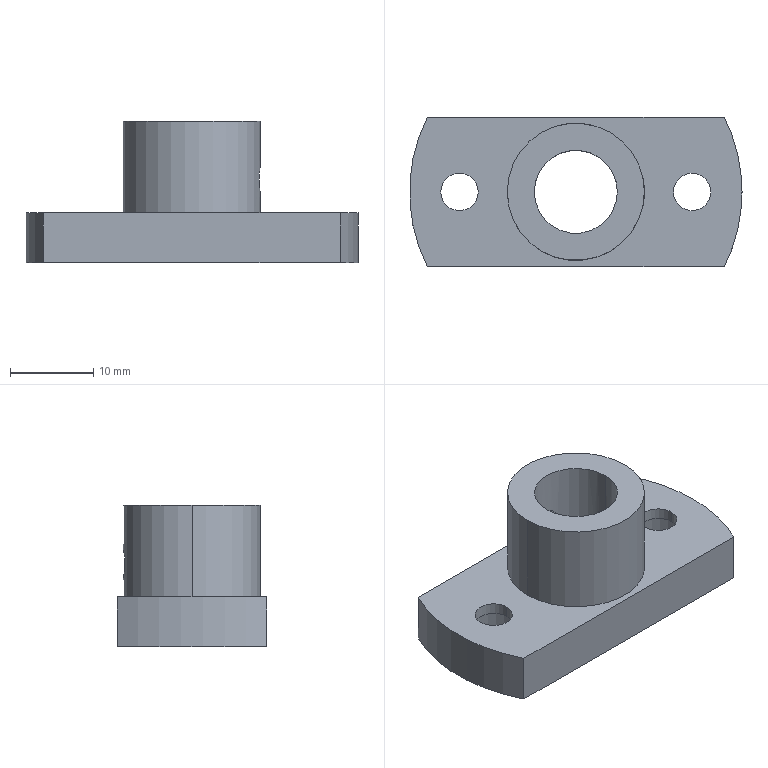Part | STEP file | Micrometer head fixing seat new | 1 solid | 26 faces | box 40 x 18 x 17 mm | volume 4623 mm3 | cylinder 19 | plane 7 | commonest cylinder face diameters 3.3 x4 4.5 x4 8 x4 40 x3 10 x2 16.5 x2
STEP:
#1=CARTESIAN_POINT('',(8.25,0.,8.35));
#2=VERTEX_POINT('',#1);
#3=CARTESIAN_POINT('',(8.25,0.,11.65));
#4=VERTEX_POINT('',#3);
#5=CARTESIAN_POINT('',(8.25,0.,8.35));
#6=CARTESIAN_POINT('',(8.25,-0.2156,8.35));
#7=CARTESIAN_POINT('',(8.241,-0.4332,8.393));
#8=CARTESIAN_POINT('',(8.218,-0.7312,8.517));
#9=CARTESIAN_POINT('',(8.209,-0.8275,8.568));
#10=CARTESIAN_POINT('',(8.189,-1.007,8.689));
#11=CARTESIAN_POINT('',(8.178,-1.09,8.757));
#12=CARTESIAN_POINT('',(8.156,-1.242,8.909));
#13=CARTESIAN_POINT('',(8.145,-1.312,8.993));
#14=CARTESIAN_POINT('',(8.125,-1.431,9.172));
#15=CARTESIAN_POINT('',(8.116,-1.482,9.266));
#16=CARTESIAN_POINT('',(8.092,-1.607,9.567));
#17=CARTESIAN_POINT('',(8.083,-1.65,9.781));
#18=CARTESIAN_POINT('',(8.083,-1.65,10.108));
#19=CARTESIAN_POINT('',(8.085,-1.639,10.215));
#20=CARTESIAN_POINT('',(8.094,-1.597,10.427));
#21=CARTESIAN_POINT('',(8.1,-1.566,10.532));
#22=CARTESIAN_POINT('',(8.116,-1.483,10.731));
#23=CARTESIAN_POINT('',(8.125,-1.432,10.826));
#24=CARTESIAN_POINT('',(8.145,-1.312,11.006));
#25=CARTESIAN_POINT('',(8.156,-1.243,11.09));
#26=CARTESIAN_POINT('',(8.189,-1.016,11.318));
#27=CARTESIAN_POINT('',(8.21,-0.8324,11.441));
#28=CARTESIAN_POINT('',(8.241,-0.4356,11.606));
#29=CARTESIAN_POINT('',(8.25,-0.2186,11.65));
#30=CARTESIAN_POINT('',(8.25,0.,11.65));
#31=B_SPLINE_CURVE_WITH_KNOTS('',3,(#5,#6,#7,#8,#9,#10,#11,#12,#13,#14,#15,#16,#17,#18,#19,#20,#21,#22,#23,#24,#25,#26,#27,#28,#29,#30),.UNSPECIFIED.,.F.,.F.,(4,2,2,2,2,2,2,2,2,2,2,2,4),(0.005172,0.005818,0.006141,0.006464,0.006787,0.007111,0.007757,0.00808,0.008403,0.008726,0.009049,0.009696,0.01034),.UNSPECIFIED.);
#32=EDGE_CURVE('',#2,#4,#31,.T.);
#33=ORIENTED_EDGE('',*,*,#32,.F.);
#34=CARTESIAN_POINT('',(5.,0.,8.35));
#35=VERTEX_POINT('',#34);
#36=CARTESIAN_POINT('',(0.,0.,8.35));
#37=DIRECTION('',(-1.,0.,0.));
#38=VECTOR('',#37,1000.);
#39=LINE('',#36,#38);
#40=EDGE_CURVE('',#2,#35,#39,.T.);
#41=ORIENTED_EDGE('',*,*,#40,.T.);
#42=CARTESIAN_POINT('',(5.,0.,11.65));
#43=VERTEX_POINT('',#42);
#44=CARTESIAN_POINT('',(5.,0.,11.65));
#45=CARTESIAN_POINT('',(5.,-0.1098,11.65));
#46=CARTESIAN_POINT('',(4.996,-0.2177,11.639));
#47=CARTESIAN_POINT('',(4.983,-0.4297,11.597));
#48=CARTESIAN_POINT('',(4.972,-0.5349,11.565));
#49=CARTESIAN_POINT('',(4.947,-0.7344,11.481));
#50=CARTESIAN_POINT('',(4.932,-0.8289,11.431));
#51=CARTESIAN_POINT('',(4.898,-1.008,11.311));
#52=CARTESIAN_POINT('',(4.88,-1.092,11.242));
#53=CARTESIAN_POINT('',(4.826,-1.318,11.015));
#54=CARTESIAN_POINT('',(4.789,-1.441,10.832));
#55=CARTESIAN_POINT('',(4.749,-1.565,10.535));
#56=CARTESIAN_POINT('',(4.738,-1.597,10.43));
#57=CARTESIAN_POINT('',(4.724,-1.639,10.217));
#58=CARTESIAN_POINT('',(4.72,-1.65,10.109));
#59=CARTESIAN_POINT('',(4.72,-1.65,9.892));
#60=CARTESIAN_POINT('',(4.724,-1.639,9.782));
#61=CARTESIAN_POINT('',(4.738,-1.597,9.57));
#62=CARTESIAN_POINT('',(4.749,-1.565,9.467));
#63=CARTESIAN_POINT('',(4.789,-1.44,9.165));
#64=CARTESIAN_POINT('',(4.826,-1.318,8.985));
#65=CARTESIAN_POINT('',(4.88,-1.09,8.757));
#66=CARTESIAN_POINT('',(4.898,-1.008,8.689));
#67=CARTESIAN_POINT('',(4.932,-0.8295,8.57));
#68=CARTESIAN_POINT('',(4.947,-0.7329,8.518));
#69=CARTESIAN_POINT('',(4.972,-0.5342,8.435));
#70=CARTESIAN_POINT('',(4.983,-0.4312,8.404));
#71=CARTESIAN_POINT('',(4.996,-0.2176,8.361));
#72=CARTESIAN_POINT('',(5.,-0.1082,8.35));
#73=CARTESIAN_POINT('',(5.,0.,8.35));
#74=B_SPLINE_CURVE_WITH_KNOTS('',3,(#44,#45,#46,#47,#48,#49,#50,#51,#52,#53,#54,#55,#56,#57,#58,#59,#60,#61,#62,#63,#64,#65,#66,#67,#68,#69,#70,#71,#72,#73),.UNSPECIFIED.,.F.,.F.,(4,2,2,2,2,2,2,2,2,2,2,2,2,2,4),(0.,0.0003247,0.0006494,0.0009741,0.001299,0.001948,0.002273,0.002598,0.002922,0.003247,0.003896,0.004221,0.004546,0.004871,0.005195),.UNSPECIFIED.);
#75=EDGE_CURVE('',#43,#35,#74,.T.);
#76=ORIENTED_EDGE('',*,*,#75,.F.);
#77=CARTESIAN_POINT('',(0.,0.,11.65));
#78=DIRECTION('',(-1.,0.,0.));
#79=VECTOR('',#78,1000.);
#80=LINE('',#77,#79);
#81=EDGE_CURVE('',#4,#43,#80,.T.);
#82=ORIENTED_EDGE('',*,*,#81,.F.);
#83=EDGE_LOOP('',(#33,#41,#76,#82));
#84=FACE_OUTER_BOUND('',#83,.T.);
#85=CARTESIAN_POINT('',(0.,0.,10.));
#86=DIRECTION('',(-1.,0.,0.));
#87=DIRECTION('',(0.,0.,1.));
#88=AXIS2_PLACEMENT_3D('',#85,#86,#87);
#89=CYLINDRICAL_SURFACE('',#88,1.65);
#90=ADVANCED_FACE('',(#84),#89,.F.);
#91=CARTESIAN_POINT('',(0.,5.,8.35));
#92=VERTEX_POINT('',#91);
#93=CARTESIAN_POINT('',(0.,5.,11.65));
#94=VERTEX_POINT('',#93);
#95=CARTESIAN_POINT('',(0.,5.,8.35));
#96=CARTESIAN_POINT('',(-0.2164,5.,8.35));
#97=CARTESIAN_POINT('',(-0.4348,4.985,8.394));
#98=CARTESIAN_POINT('',(-0.7334,4.947,8.518));
#99=CARTESIAN_POINT('',(-0.8299,4.931,8.57));
#100=CARTESIAN_POINT('',(-1.008,4.898,8.689));
#101=CARTESIAN_POINT('',(-1.091,4.88,8.757));
#102=CARTESIAN_POINT('',(-1.319,4.825,8.986));
#103=CARTESIAN_POINT('',(-1.44,4.789,9.166));
#104=CARTESIAN_POINT('',(-1.565,4.749,9.467));
#105=CARTESIAN_POINT('',(-1.597,4.738,9.57));
#106=CARTESIAN_POINT('',(-1.639,4.724,9.781));
#107=CARTESIAN_POINT('',(-1.65,4.72,9.891));
#108=CARTESIAN_POINT('',(-1.65,4.72,10.109));
#109=CARTESIAN_POINT('',(-1.639,4.724,10.217));
#110=CARTESIAN_POINT('',(-1.597,4.738,10.43));
#111=CARTESIAN_POINT('',(-1.565,4.749,10.535));
#112=CARTESIAN_POINT('',(-1.441,4.789,10.833));
#113=CARTESIAN_POINT('',(-1.318,4.826,11.015));
#114=CARTESIAN_POINT('',(-1.091,4.88,11.242));
#115=CARTESIAN_POINT('',(-1.007,4.898,11.311));
#116=CARTESIAN_POINT('',(-0.8287,4.932,11.431));
#117=CARTESIAN_POINT('',(-0.7344,4.947,11.481));
#118=CARTESIAN_POINT('',(-0.535,4.972,11.565));
#119=CARTESIAN_POINT('',(-0.4297,4.983,11.597));
#120=CARTESIAN_POINT('',(-0.2177,4.996,11.639));
#121=CARTESIAN_POINT('',(-0.1098,5.,11.65));
#122=CARTESIAN_POINT('',(0.,5.,11.65));
#123=B_SPLINE_CURVE_WITH_KNOTS('',3,(#95,#96,#97,#98,#99,#100,#101,#102,#103,#104,#105,#106,#107,#108,#109,#110,#111,#112,#113,#114,#115,#116,#117,#118,#119,#120,#121,#122),.UNSPECIFIED.,.F.,.F.,(4,2,2,2,2,2,2,2,2,2,2,2,2,4),(0.005195,0.005845,0.006169,0.006494,0.007143,0.007468,0.007792,0.008117,0.008442,0.009091,0.009415,0.00974,0.01006,0.01039),.UNSPECIFIED.);
#124=EDGE_CURVE('',#92,#94,#123,.T.);
#125=ORIENTED_EDGE('',*,*,#124,.F.);
#126=CARTESIAN_POINT('',(0.,8.25,8.35));
#127=VERTEX_POINT('',#126);
#128=CARTESIAN_POINT('',(0.,9.,8.35));
#129=DIRECTION('',(0.,1.,0.));
#130=VECTOR('',#129,1000.);
#131=LINE('',#128,#130);
#132=EDGE_CURVE('',#92,#127,#131,.T.);
#133=ORIENTED_EDGE('',*,*,#132,.T.);
#134=CARTESIAN_POINT('',(0.,8.25,11.65));
#135=VERTEX_POINT('',#134);
#136=CARTESIAN_POINT('',(0.,8.25,11.65));
#137=CARTESIAN_POINT('',(-0.1093,8.25,11.65));
#138=CARTESIAN_POINT('',(-0.2168,8.248,11.639));
#139=CARTESIAN_POINT('',(-0.428,8.24,11.597));
#140=CARTESIAN_POINT('',(-0.533,8.233,11.565));
#141=CARTESIAN_POINT('',(-0.7327,8.218,11.482));
#142=CARTESIAN_POINT('',(-0.8274,8.209,11.432));
#143=CARTESIAN_POINT('',(-1.007,8.189,11.312));
#144=CARTESIAN_POINT('',(-1.091,8.178,11.242));
#145=CARTESIAN_POINT('',(-1.319,8.145,11.015));
#146=CARTESIAN_POINT('',(-1.442,8.124,10.831));
#147=CARTESIAN_POINT('',(-1.606,8.093,10.434));
#148=CARTESIAN_POINT('',(-1.65,8.083,10.216));
#149=CARTESIAN_POINT('',(-1.65,8.083,9.893));
#150=CARTESIAN_POINT('',(-1.639,8.086,9.783));
#151=CARTESIAN_POINT('',(-1.597,8.094,9.571));
#152=CARTESIAN_POINT('',(-1.566,8.1,9.468));
#153=CARTESIAN_POINT('',(-1.441,8.124,9.168));
#154=CARTESIAN_POINT('',(-1.32,8.145,8.987));
#155=CARTESIAN_POINT('',(-1.09,8.178,8.757));
#156=CARTESIAN_POINT('',(-1.007,8.189,8.688));
#157=CARTESIAN_POINT('',(-0.8284,8.209,8.569));
#158=CARTESIAN_POINT('',(-0.7318,8.218,8.517));
#159=CARTESIAN_POINT('',(-0.5323,8.233,8.435));
#160=CARTESIAN_POINT('',(-0.4295,8.239,8.403));
#161=CARTESIAN_POINT('',(-0.2174,8.248,8.361));
#162=CARTESIAN_POINT('',(-0.1078,8.25,8.35));
#163=CARTESIAN_POINT('',(0.,8.25,8.35));
#164=B_SPLINE_CURVE_WITH_KNOTS('',3,(#136,#137,#138,#139,#140,#141,#142,#143,#144,#145,#146,#147,#148,#149,#150,#151,#152,#153,#154,#155,#156,#157,#158,#159,#160,#161,#162,#163),.UNSPECIFIED.,.F.,.F.,(4,2,2,2,2,2,2,2,2,2,2,2,2,4),(0.,0.0003232,0.0006465,0.0009697,0.001293,0.001939,0.002586,0.002909,0.003232,0.003879,0.004202,0.004525,0.004848,0.005172),.UNSPECIFIED.);
#165=EDGE_CURVE('',#135,#127,#164,.T.);
#166=ORIENTED_EDGE('',*,*,#165,.F.);
#167=CARTESIAN_POINT('',(0.,9.,11.65));
#168=DIRECTION('',(0.,1.,0.));
#169=VECTOR('',#168,1000.);
#170=LINE('',#167,#169);
#171=EDGE_CURVE('',#94,#135,#170,.T.);
#172=ORIENTED_EDGE('',*,*,#171,.F.);
#173=EDGE_LOOP('',(#125,#133,#166,#172));
#174=FACE_OUTER_BOUND('',#173,.T.);
#175=CARTESIAN_POINT('',(0.,9.,10.));
#176=DIRECTION('',(0.,1.,0.));
#177=DIRECTION('',(0.,0.,1.));
#178=AXIS2_PLACEMENT_3D('',#175,#176,#177);
#179=CYLINDRICAL_SURFACE('',#178,1.65);
#180=ADVANCED_FACE('',(#174),#179,.F.);
#181=CARTESIAN_POINT('',(18.,0.,4.6));
#182=VERTEX_POINT('',#181);
#183=CARTESIAN_POINT('',(10.,0.,4.6));
#184=VERTEX_POINT('',#183);
#185=CARTESIAN_POINT('',(14.,0.,4.6));
#186=DIRECTION('',(0.,0.,-1.));
#187=DIRECTION('',(-1.,0.,0.));
#188=AXIS2_PLACEMENT_3D('',#185,#186,#187);
#189=CIRCLE('',#188,4.);
#190=EDGE_CURVE('',#182,#184,#189,.T.);
#191=ORIENTED_EDGE('',*,*,#190,.F.);
#192=CARTESIAN_POINT('',(18.,0.,0.));
#193=VERTEX_POINT('',#192);
#194=CARTESIAN_POINT('',(18.,0.,0.));
#195=DIRECTION('',(0.,0.,-1.));
#196=VECTOR('',#195,1000.);
#197=LINE('',#194,#196);
#198=EDGE_CURVE('',#182,#193,#197,.T.);
#199=ORIENTED_EDGE('',*,*,#198,.T.);
#200=CARTESIAN_POINT('',(10.,0.,0.));
#201=VERTEX_POINT('',#200);
#202=CARTESIAN_POINT('',(14.,0.,0.));
#203=DIRECTION('',(0.,0.,-1.));
#204=DIRECTION('',(-1.,0.,0.));
#205=AXIS2_PLACEMENT_3D('',#202,#203,#204);
#206=CIRCLE('',#205,4.);
#207=EDGE_CURVE('',#193,#201,#206,.T.);
#208=ORIENTED_EDGE('',*,*,#207,.T.);
#209=CARTESIAN_POINT('',(10.,0.,0.));
#210=DIRECTION('',(0.,0.,-1.));
#211=VECTOR('',#210,1000.);
#212=LINE('',#209,#211);
#213=EDGE_CURVE('',#184,#201,#212,.T.);
#214=ORIENTED_EDGE('',*,*,#213,.F.);
#215=EDGE_LOOP('',(#191,#199,#208,#214));
#216=FACE_OUTER_BOUND('',#215,.T.);
#217=CARTESIAN_POINT('',(14.,0.,0.));
#218=DIRECTION('',(0.,0.,-1.));
#219=DIRECTION('',(-1.,0.,0.));
#220=AXIS2_PLACEMENT_3D('',#217,#218,#219);
#221=CYLINDRICAL_SURFACE('',#220,4.);
#222=ADVANCED_FACE('',(#216),#221,.F.);
#223=CARTESIAN_POINT('',(11.75,0.,6.));
#224=VERTEX_POINT('',#223);
#225=CARTESIAN_POINT('',(16.25,0.,6.));
#226=VERTEX_POINT('',#225);
#227=CARTESIAN_POINT('',(14.,0.,6.));
#228=DIRECTION('',(0.,0.,1.));
#229=DIRECTION('',(1.,0.,0.));
#230=AXIS2_PLACEMENT_3D('',#227,#228,#229);
#231=CIRCLE('',#230,2.25);
#232=EDGE_CURVE('',#224,#226,#231,.T.);
#233=ORIENTED_EDGE('',*,*,#232,.T.);
#234=CARTESIAN_POINT('',(16.25,0.,4.6));
#235=VERTEX_POINT('',#234);
#236=CARTESIAN_POINT('',(16.25,0.,0.));
#237=DIRECTION('',(0.,0.,-1.));
#238=VECTOR('',#237,1000.);
#239=LINE('',#236,#238);
#240=EDGE_CURVE('',#226,#235,#239,.T.);
#241=ORIENTED_EDGE('',*,*,#240,.T.);
#242=CARTESIAN_POINT('',(11.75,0.,4.6));
#243=VERTEX_POINT('',#242);
#244=CARTESIAN_POINT('',(14.,0.,4.6));
#245=DIRECTION('',(0.,0.,-1.));
#246=DIRECTION('',(-1.,0.,0.));
#247=AXIS2_PLACEMENT_3D('',#244,#245,#246);
#248=CIRCLE('',#247,2.25);
#249=EDGE_CURVE('',#235,#243,#248,.T.);
#250=ORIENTED_EDGE('',*,*,#249,.T.);
#251=CARTESIAN_POINT('',(11.75,0.,0.));
#252=DIRECTION('',(0.,0.,-1.));
#253=VECTOR('',#252,1000.);
#254=LINE('',#251,#253);
#255=EDGE_CURVE('',#224,#243,#254,.T.);
#256=ORIENTED_EDGE('',*,*,#255,.F.);
#257=EDGE_LOOP('',(#233,#241,#250,#256));
#258=FACE_OUTER_BOUND('',#257,.T.);
#259=CARTESIAN_POINT('',(14.,0.,0.));
#260=DIRECTION('',(0.,0.,-1.));
#261=DIRECTION('',(-1.,0.,0.));
#262=AXIS2_PLACEMENT_3D('',#259,#260,#261);
#263=CYLINDRICAL_SURFACE('',#262,2.25);
#264=ADVANCED_FACE('',(#258),#263,.F.);
#265=CARTESIAN_POINT('',(-10.,0.,4.6));
#266=VERTEX_POINT('',#265);
#267=CARTESIAN_POINT('',(-18.,0.,4.6));
#268=VERTEX_POINT('',#267);
#269=CARTESIAN_POINT('',(-14.,0.,4.6));
#270=DIRECTION('',(0.,0.,-1.));
#271=DIRECTION('',(-1.,0.,0.));
#272=AXIS2_PLACEMENT_3D('',#269,#270,#271);
#273=CIRCLE('',#272,4.);
#274=EDGE_CURVE('',#266,#268,#273,.T.);
#275=ORIENTED_EDGE('',*,*,#274,.F.);
#276=CARTESIAN_POINT('',(-10.,0.,0.));
#277=VERTEX_POINT('',#276);
#278=CARTESIAN_POINT('',(-10.,0.,0.));
#279=DIRECTION('',(0.,0.,-1.));
#280=VECTOR('',#279,1000.);
#281=LINE('',#278,#280);
#282=EDGE_CURVE('',#266,#277,#281,.T.);
#283=ORIENTED_EDGE('',*,*,#282,.T.);
#284=CARTESIAN_POINT('',(-18.,0.,0.));
#285=VERTEX_POINT('',#284);
#286=CARTESIAN_POINT('',(-14.,0.,0.));
#287=DIRECTION('',(0.,0.,-1.));
#288=DIRECTION('',(-1.,0.,0.));
#289=AXIS2_PLACEMENT_3D('',#286,#287,#288);
#290=CIRCLE('',#289,4.);
#291=EDGE_CURVE('',#277,#285,#290,.T.);
#292=ORIENTED_EDGE('',*,*,#291,.T.);
#293=CARTESIAN_POINT('',(-18.,0.,0.));
#294=DIRECTION('',(0.,0.,-1.));
#295=VECTOR('',#294,1000.);
#296=LINE('',#293,#295);
#297=EDGE_CURVE('',#268,#285,#296,.T.);
#298=ORIENTED_EDGE('',*,*,#297,.F.);
#299=EDGE_LOOP('',(#275,#283,#292,#298));
#300=FACE_OUTER_BOUND('',#299,.T.);
#301=CARTESIAN_POINT('',(-14.,0.,0.));
#302=DIRECTION('',(0.,0.,-1.));
#303=DIRECTION('',(-1.,0.,0.));
#304=AXIS2_PLACEMENT_3D('',#301,#302,#303);
#305=CYLINDRICAL_SURFACE('',#304,4.);
#306=ADVANCED_FACE('',(#300),#305,.F.);
#307=CARTESIAN_POINT('',(-16.25,0.,6.));
#308=VERTEX_POINT('',#307);
#309=CARTESIAN_POINT('',(-11.75,0.,6.));
#310=VERTEX_POINT('',#309);
#311=CARTESIAN_POINT('',(-14.,0.,6.));
#312=DIRECTION('',(0.,0.,1.));
#313=DIRECTION('',(1.,0.,0.));
#314=AXIS2_PLACEMENT_3D('',#311,#312,#313);
#315=CIRCLE('',#314,2.25);
#316=EDGE_CURVE('',#308,#310,#315,.T.);
#317=ORIENTED_EDGE('',*,*,#316,.T.);
#318=CARTESIAN_POINT('',(-11.75,0.,4.6));
#319=VERTEX_POINT('',#318);
#320=CARTESIAN_POINT('',(-11.75,0.,0.));
#321=DIRECTION('',(0.,0.,-1.));
#322=VECTOR('',#321,1000.);
#323=LINE('',#320,#322);
#324=EDGE_CURVE('',#310,#319,#323,.T.);
#325=ORIENTED_EDGE('',*,*,#324,.T.);
#326=CARTESIAN_POINT('',(-16.25,0.,4.6));
#327=VERTEX_POINT('',#326);
#328=CARTESIAN_POINT('',(-14.,0.,4.6));
#329=DIRECTION('',(0.,0.,-1.));
#330=DIRECTION('',(-1.,0.,0.));
#331=AXIS2_PLACEMENT_3D('',#328,#329,#330);
#332=CIRCLE('',#331,2.25);
#333=EDGE_CURVE('',#319,#327,#332,.T.);
#334=ORIENTED_EDGE('',*,*,#333,.T.);
#335=CARTESIAN_POINT('',(-16.25,0.,0.));
#336=DIRECTION('',(0.,0.,-1.));
#337=VECTOR('',#336,1000.);
#338=LINE('',#335,#337);
#339=EDGE_CURVE('',#308,#327,#338,.T.);
#340=ORIENTED_EDGE('',*,*,#339,.F.);
#341=EDGE_LOOP('',(#317,#325,#334,#340));
#342=FACE_OUTER_BOUND('',#341,.T.);
#343=CARTESIAN_POINT('',(-14.,0.,0.));
#344=DIRECTION('',(0.,0.,-1.));
#345=DIRECTION('',(-1.,0.,0.));
#346=AXIS2_PLACEMENT_3D('',#343,#344,#345);
#347=CYLINDRICAL_SURFACE('',#346,2.25);
#348=ADVANCED_FACE('',(#342),#347,.F.);
#349=CARTESIAN_POINT('',(5.,0.,17.));
#350=VERTEX_POINT('',#349);
#351=CARTESIAN_POINT('',(-5.,0.,17.));
#352=VERTEX_POINT('',#351);
#353=CARTESIAN_POINT('',(0.,0.,17.));
#354=DIRECTION('',(0.,0.,-1.));
#355=DIRECTION('',(-1.,0.,0.));
#356=AXIS2_PLACEMENT_3D('',#353,#354,#355);
#357=CIRCLE('',#356,5.);
#358=EDGE_CURVE('',#350,#352,#357,.T.);
#359=ORIENTED_EDGE('',*,*,#358,.F.);
#360=CARTESIAN_POINT('',(5.,0.,17.));
#361=DIRECTION('',(0.,0.,-1.));
#362=VECTOR('',#361,1000.);
#363=LINE('',#360,#362);
#364=EDGE_CURVE('',#350,#43,#363,.T.);
#365=ORIENTED_EDGE('',*,*,#364,.T.);
#366=ORIENTED_EDGE('',*,*,#75,.T.);
#367=CARTESIAN_POINT('',(5.,0.,0.));
#368=VERTEX_POINT('',#367);
#369=CARTESIAN_POINT('',(5.,0.,17.));
#370=DIRECTION('',(0.,0.,-1.));
#371=VECTOR('',#370,1000.);
#372=LINE('',#369,#371);
#373=EDGE_CURVE('',#35,#368,#372,.T.);
#374=ORIENTED_EDGE('',*,*,#373,.T.);
#375=CARTESIAN_POINT('',(-5.,0.,0.));
#376=VERTEX_POINT('',#375);
#377=CARTESIAN_POINT('',(0.,0.,0.));
#378=DIRECTION('',(0.,0.,-1.));
#379=DIRECTION('',(-1.,0.,0.));
#380=AXIS2_PLACEMENT_3D('',#377,#378,#379);
#381=CIRCLE('',#380,5.);
#382=EDGE_CURVE('',#368,#376,#381,.T.);
#383=ORIENTED_EDGE('',*,*,#382,.T.);
#384=CARTESIAN_POINT('',(-5.,0.,17.));
#385=DIRECTION('',(0.,0.,-1.));
#386=VECTOR('',#385,1000.);
#387=LINE('',#384,#386);
#388=EDGE_CURVE('',#352,#376,#387,.T.);
#389=ORIENTED_EDGE('',*,*,#388,.F.);
#390=EDGE_LOOP('',(#359,#365,#366,#374,#383,#389));
#391=FACE_OUTER_BOUND('',#390,.T.);
#392=CARTESIAN_POINT('',(0.,0.,17.));
#393=DIRECTION('',(0.,0.,-1.));
#394=DIRECTION('',(-1.,0.,0.));
#395=AXIS2_PLACEMENT_3D('',#392,#393,#394);
#396=CYLINDRICAL_SURFACE('',#395,5.);
#397=ADVANCED_FACE('',(#391),#396,.F.);
#398=ORIENTED_EDGE('',*,*,#165,.T.);
#399=CARTESIAN_POINT('',(0.,8.25,8.35));
#400=CARTESIAN_POINT('',(0.2156,8.25,8.35));
#401=CARTESIAN_POINT('',(0.4332,8.241,8.393));
#402=CARTESIAN_POINT('',(0.7312,8.218,8.517));
#403=CARTESIAN_POINT('',(0.8275,8.209,8.568));
#404=CARTESIAN_POINT('',(1.007,8.189,8.689));
#405=CARTESIAN_POINT('',(1.09,8.178,8.757));
#406=CARTESIAN_POINT('',(1.242,8.156,8.909));
#407=CARTESIAN_POINT('',(1.312,8.145,8.993));
#408=CARTESIAN_POINT('',(1.431,8.125,9.172));
#409=CARTESIAN_POINT('',(1.482,8.116,9.266));
#410=CARTESIAN_POINT('',(1.607,8.092,9.567));
#411=CARTESIAN_POINT('',(1.65,8.083,9.781));
#412=CARTESIAN_POINT('',(1.65,8.083,10.108));
#413=CARTESIAN_POINT('',(1.639,8.085,10.215));
#414=CARTESIAN_POINT('',(1.597,8.094,10.427));
#415=CARTESIAN_POINT('',(1.566,8.1,10.532));
#416=CARTESIAN_POINT('',(1.483,8.116,10.731));
#417=CARTESIAN_POINT('',(1.432,8.125,10.826));
#418=CARTESIAN_POINT('',(1.312,8.145,11.006));
#419=CARTESIAN_POINT('',(1.243,8.156,11.09));
#420=CARTESIAN_POINT('',(1.016,8.189,11.318));
#421=CARTESIAN_POINT('',(0.8324,8.21,11.441));
#422=CARTESIAN_POINT('',(0.4356,8.241,11.606));
#423=CARTESIAN_POINT('',(0.2186,8.25,11.65));
#424=CARTESIAN_POINT('',(0.,8.25,11.65));
#425=B_SPLINE_CURVE_WITH_KNOTS('',3,(#399,#400,#401,#402,#403,#404,#405,#406,#407,#408,#409,#410,#411,#412,#413,#414,#415,#416,#417,#418,#419,#420,#421,#422,#423,#424),.UNSPECIFIED.,.F.,.F.,(4,2,2,2,2,2,2,2,2,2,2,2,4),(0.005172,0.005818,0.006141,0.006464,0.006787,0.007111,0.007757,0.00808,0.008403,0.008726,0.009049,0.009696,0.01034),.UNSPECIFIED.);
#426=EDGE_CURVE('',#127,#135,#425,.T.);
#427=ORIENTED_EDGE('',*,*,#426,.T.);
#428=EDGE_LOOP('',(#398,#427));
#429=FACE_BOUND('',#428,.T.);
#430=CARTESIAN_POINT('',(8.25,0.,17.));
#431=VERTEX_POINT('',#430);
#432=CARTESIAN_POINT('',(-8.25,0.,17.));
#433=VERTEX_POINT('',#432);
#434=CARTESIAN_POINT('',(0.,0.,17.));
#435=DIRECTION('',(0.,0.,1.));
#436=DIRECTION('',(1.,0.,0.));
#437=AXIS2_PLACEMENT_3D('',#434,#435,#436);
#438=CIRCLE('',#437,8.25);
#439=EDGE_CURVE('',#431,#433,#438,.T.);
#440=ORIENTED_EDGE('',*,*,#439,.F.);
#441=CARTESIAN_POINT('',(8.25,0.,17.));
#442=DIRECTION('',(0.,0.,-1.));
#443=VECTOR('',#442,1000.);
#444=LINE('',#441,#443);
#445=EDGE_CURVE('',#431,#4,#444,.T.);
#446=ORIENTED_EDGE('',*,*,#445,.T.);
#447=CARTESIAN_POINT('',(8.25,0.,11.65));
#448=CARTESIAN_POINT('',(8.25,0.1093,11.65));
#449=CARTESIAN_POINT('',(8.248,0.2168,11.639));
#450=CARTESIAN_POINT('',(8.24,0.428,11.597));
#451=CARTESIAN_POINT('',(8.233,0.533,11.565));
#452=CARTESIAN_POINT('',(8.218,0.7327,11.482));
#453=CARTESIAN_POINT('',(8.209,0.8274,11.432));
#454=CARTESIAN_POINT('',(8.189,1.007,11.312));
#455=CARTESIAN_POINT('',(8.178,1.091,11.242));
#456=CARTESIAN_POINT('',(8.145,1.319,11.015));
#457=CARTESIAN_POINT('',(8.124,1.442,10.831));
#458=CARTESIAN_POINT('',(8.093,1.606,10.434));
#459=CARTESIAN_POINT('',(8.083,1.65,10.216));
#460=CARTESIAN_POINT('',(8.083,1.65,9.893));
#461=CARTESIAN_POINT('',(8.086,1.639,9.783));
#462=CARTESIAN_POINT('',(8.094,1.597,9.571));
#463=CARTESIAN_POINT('',(8.1,1.566,9.468));
#464=CARTESIAN_POINT('',(8.124,1.441,9.168));
#465=CARTESIAN_POINT('',(8.145,1.32,8.987));
#466=CARTESIAN_POINT('',(8.178,1.09,8.757));
#467=CARTESIAN_POINT('',(8.189,1.007,8.688));
#468=CARTESIAN_POINT('',(8.209,0.8284,8.569));
#469=CARTESIAN_POINT('',(8.218,0.7318,8.517));
#470=CARTESIAN_POINT('',(8.233,0.5323,8.435));
#471=CARTESIAN_POINT('',(8.239,0.4295,8.403));
#472=CARTESIAN_POINT('',(8.248,0.2174,8.361));
#473=CARTESIAN_POINT('',(8.25,0.1078,8.35));
#474=CARTESIAN_POINT('',(8.25,0.,8.35));
#475=B_SPLINE_CURVE_WITH_KNOTS('',3,(#447,#448,#449,#450,#451,#452,#453,#454,#455,#456,#457,#458,#459,#460,#461,#462,#463,#464,#465,#466,#467,#468,#469,#470,#471,#472,#473,#474),.UNSPECIFIED.,.F.,.F.,(4,2,2,2,2,2,2,2,2,2,2,2,2,4),(0.,0.0003232,0.0006465,0.0009697,0.001293,0.001939,0.002586,0.002909,0.003232,0.003879,0.004202,0.004525,0.004848,0.005172),.UNSPECIFIED.);
#476=EDGE_CURVE('',#4,#2,#475,.T.);
#477=ORIENTED_EDGE('',*,*,#476,.T.);
#478=CARTESIAN_POINT('',(8.25,0.,6.));
#479=VERTEX_POINT('',#478);
#480=CARTESIAN_POINT('',(8.25,0.,17.));
#481=DIRECTION('',(0.,0.,-1.));
#482=VECTOR('',#481,1000.);
#483=LINE('',#480,#482);
#484=EDGE_CURVE('',#2,#479,#483,.T.);
#485=ORIENTED_EDGE('',*,*,#484,.T.);
#486=CARTESIAN_POINT('',(-8.25,0.,6.));
#487=VERTEX_POINT('',#486);
#488=CARTESIAN_POINT('',(0.,0.,6.));
#489=DIRECTION('',(0.,0.,1.));
#490=DIRECTION('',(1.,0.,0.));
#491=AXIS2_PLACEMENT_3D('',#488,#489,#490);
#492=CIRCLE('',#491,8.25);
#493=EDGE_CURVE('',#479,#487,#492,.T.);
#494=ORIENTED_EDGE('',*,*,#493,.T.);
#495=CARTESIAN_POINT('',(-8.25,0.,17.));
#496=DIRECTION('',(0.,0.,-1.));
#497=VECTOR('',#496,1000.);
#498=LINE('',#495,#497);
#499=EDGE_CURVE('',#433,#487,#498,.T.);
#500=ORIENTED_EDGE('',*,*,#499,.F.);
#501=EDGE_LOOP('',(#440,#446,#477,#485,#494,#500));
#502=FACE_OUTER_BOUND('',#501,.T.);
#503=CARTESIAN_POINT('',(0.,0.,17.));
#504=DIRECTION('',(0.,0.,-1.));
#505=DIRECTION('',(-1.,0.,0.));
#506=AXIS2_PLACEMENT_3D('',#503,#504,#505);
#507=CYLINDRICAL_SURFACE('',#506,8.25);
#508=ADVANCED_FACE('',(#429,#502),#507,.T.);
#509=CARTESIAN_POINT('',(17.861,-9.,0.));
#510=VERTEX_POINT('',#509);
#511=CARTESIAN_POINT('',(20.,0.,0.));
#512=VERTEX_POINT('',#511);
#513=CARTESIAN_POINT('',(0.,0.,0.));
#514=DIRECTION('',(0.,0.,1.));
#515=DIRECTION('',(1.,0.,0.));
#516=AXIS2_PLACEMENT_3D('',#513,#514,#515);
#517=CIRCLE('',#516,20.);
#518=EDGE_CURVE('',#510,#512,#517,.T.);
#519=ORIENTED_EDGE('',*,*,#518,.T.);
#520=CARTESIAN_POINT('',(20.,0.,6.));
#521=VERTEX_POINT('',#520);
#522=CARTESIAN_POINT('',(20.,0.,0.));
#523=DIRECTION('',(0.,0.,1.));
#524=VECTOR('',#523,1000.);
#525=LINE('',#522,#524);
#526=EDGE_CURVE('',#512,#521,#525,.T.);
#527=ORIENTED_EDGE('',*,*,#526,.T.);
#528=CARTESIAN_POINT('',(17.861,-9.,6.));
#529=VERTEX_POINT('',#528);
#530=CARTESIAN_POINT('',(0.,0.,6.));
#531=DIRECTION('',(0.,0.,1.));
#532=DIRECTION('',(1.,0.,0.));
#533=AXIS2_PLACEMENT_3D('',#530,#531,#532);
#534=CIRCLE('',#533,20.);
#535=EDGE_CURVE('',#529,#521,#534,.T.);
#536=ORIENTED_EDGE('',*,*,#535,.F.);
#537=CARTESIAN_POINT('',(17.861,-9.,0.));
#538=DIRECTION('',(0.,0.,-1.));
#539=VECTOR('',#538,1000.);
#540=LINE('',#537,#539);
#541=EDGE_CURVE('',#529,#510,#540,.T.);
#542=ORIENTED_EDGE('',*,*,#541,.T.);
#543=EDGE_LOOP('',(#519,#527,#536,#542));
#544=FACE_OUTER_BOUND('',#543,.T.);
#545=CARTESIAN_POINT('',(0.,0.,0.));
#546=DIRECTION('',(0.,0.,1.));
#547=DIRECTION('',(1.,0.,0.));
#548=AXIS2_PLACEMENT_3D('',#545,#546,#547);
#549=CYLINDRICAL_SURFACE('',#548,20.);
#550=ADVANCED_FACE('',(#544),#549,.T.);
#551=ORIENTED_EDGE('',*,*,#232,.F.);
#552=CARTESIAN_POINT('',(14.,0.,6.));
#553=DIRECTION('',(0.,0.,1.));
#554=DIRECTION('',(1.,0.,0.));
#555=AXIS2_PLACEMENT_3D('',#552,#553,#554);
#556=CIRCLE('',#555,2.25);
#557=EDGE_CURVE('',#226,#224,#556,.T.);
#558=ORIENTED_EDGE('',*,*,#557,.F.);
#559=EDGE_LOOP('',(#551,#558));
#560=FACE_BOUND('',#559,.T.);
#561=ORIENTED_EDGE('',*,*,#316,.F.);
#562=CARTESIAN_POINT('',(-14.,0.,6.));
#563=DIRECTION('',(0.,0.,1.));
#564=DIRECTION('',(1.,0.,0.));
#565=AXIS2_PLACEMENT_3D('',#562,#563,#564);
#566=CIRCLE('',#565,2.25);
#567=EDGE_CURVE('',#310,#308,#566,.T.);
#568=ORIENTED_EDGE('',*,*,#567,.F.);
#569=EDGE_LOOP('',(#561,#568));
#570=FACE_BOUND('',#569,.T.);
#571=CARTESIAN_POINT('',(17.861,9.,6.));
#572=VERTEX_POINT('',#571);
#573=CARTESIAN_POINT('',(-17.861,9.,6.));
#574=VERTEX_POINT('',#573);
#575=CARTESIAN_POINT('',(-40.,9.,6.));
#576=DIRECTION('',(-1.,0.,0.));
#577=VECTOR('',#576,1000.);
#578=LINE('',#575,#577);
#579=EDGE_CURVE('',#572,#574,#578,.T.);
#580=ORIENTED_EDGE('',*,*,#579,.T.);
#581=CARTESIAN_POINT('',(-17.861,-9.,6.));
#582=VERTEX_POINT('',#581);
#583=CARTESIAN_POINT('',(0.,0.,6.));
#584=DIRECTION('',(0.,0.,1.));
#585=DIRECTION('',(1.,0.,0.));
#586=AXIS2_PLACEMENT_3D('',#583,#584,#585);
#587=CIRCLE('',#586,20.);
#588=EDGE_CURVE('',#574,#582,#587,.T.);
#589=ORIENTED_EDGE('',*,*,#588,.T.);
#590=CARTESIAN_POINT('',(-40.,-9.,6.));
#591=DIRECTION('',(1.,0.,0.));
#592=VECTOR('',#591,1000.);
#593=LINE('',#590,#592);
#594=EDGE_CURVE('',#582,#529,#593,.T.);
#595=ORIENTED_EDGE('',*,*,#594,.T.);
#596=ORIENTED_EDGE('',*,*,#535,.T.);
#597=CARTESIAN_POINT('',(0.,0.,6.));
#598=DIRECTION('',(0.,0.,1.));
#599=DIRECTION('',(1.,0.,0.));
#600=AXIS2_PLACEMENT_3D('',#597,#598,#599);
#601=CIRCLE('',#600,20.);
#602=EDGE_CURVE('',#521,#572,#601,.T.);
#603=ORIENTED_EDGE('',*,*,#602,.T.);
#604=EDGE_LOOP('',(#580,#589,#595,#596,#603));
#605=FACE_OUTER_BOUND('',#604,.T.);
#606=CARTESIAN_POINT('',(0.,0.,6.));
#607=DIRECTION('',(0.,0.,1.));
#608=DIRECTION('',(1.,0.,0.));
#609=AXIS2_PLACEMENT_3D('',#606,#607,#608);
#610=CIRCLE('',#609,8.25);
#611=EDGE_CURVE('',#487,#479,#610,.T.);
#612=ORIENTED_EDGE('',*,*,#611,.F.);
#613=ORIENTED_EDGE('',*,*,#493,.F.);
#614=EDGE_LOOP('',(#612,#613));
#615=FACE_BOUND('',#614,.T.);
#616=CARTESIAN_POINT('',(0.,0.,6.));
#617=DIRECTION('',(0.,0.,1.));
#618=DIRECTION('',(1.,0.,0.));
#619=AXIS2_PLACEMENT_3D('',#616,#617,#618);
#620=PLANE('',#619);
#621=ADVANCED_FACE('',(#560,#570,#605,#615),#620,.T.);
#622=CARTESIAN_POINT('',(17.861,9.,0.));
#623=VERTEX_POINT('',#622);
#624=CARTESIAN_POINT('',(17.861,9.,0.));
#625=DIRECTION('',(0.,0.,1.));
#626=VECTOR('',#625,1000.);
#627=LINE('',#624,#626);
#628=EDGE_CURVE('',#623,#572,#627,.T.);
#629=ORIENTED_EDGE('',*,*,#628,.F.);
#630=CARTESIAN_POINT('',(-17.861,9.,0.));
#631=VERTEX_POINT('',#630);
#632=CARTESIAN_POINT('',(-40.,9.,0.));
#633=DIRECTION('',(-1.,0.,0.));
#634=VECTOR('',#633,1000.);
#635=LINE('',#632,#634);
#636=EDGE_CURVE('',#623,#631,#635,.T.);
#637=ORIENTED_EDGE('',*,*,#636,.T.);
#638=CARTESIAN_POINT('',(-17.861,9.,0.));
#639=DIRECTION('',(0.,0.,-1.));
#640=VECTOR('',#639,1000.);
#641=LINE('',#638,#640);
#642=EDGE_CURVE('',#574,#631,#641,.T.);
#643=ORIENTED_EDGE('',*,*,#642,.F.);
#644=ORIENTED_EDGE('',*,*,#579,.F.);
#645=EDGE_LOOP('',(#629,#637,#643,#644));
#646=FACE_OUTER_BOUND('',#645,.T.);
#647=CARTESIAN_POINT('',(-40.,9.,6.));
#648=DIRECTION('',(0.,-1.,0.));
#649=DIRECTION('',(0.,0.,-1.));
#650=AXIS2_PLACEMENT_3D('',#647,#648,#649);
#651=PLANE('',#650);
#652=ADVANCED_FACE('',(#646),#651,.F.);
#653=CARTESIAN_POINT('',(-17.861,-9.,0.));
#654=VERTEX_POINT('',#653);
#655=CARTESIAN_POINT('',(-17.861,-9.,0.));
#656=DIRECTION('',(0.,0.,1.));
#657=VECTOR('',#656,1000.);
#658=LINE('',#655,#657);
#659=EDGE_CURVE('',#654,#582,#658,.T.);
#660=ORIENTED_EDGE('',*,*,#659,.F.);
#661=CARTESIAN_POINT('',(-40.,-9.,0.));
#662=DIRECTION('',(1.,0.,0.));
#663=VECTOR('',#662,1000.);
#664=LINE('',#661,#663);
#665=EDGE_CURVE('',#654,#510,#664,.T.);
#666=ORIENTED_EDGE('',*,*,#665,.T.);
#667=ORIENTED_EDGE('',*,*,#541,.F.);
#668=ORIENTED_EDGE('',*,*,#594,.F.);
#669=EDGE_LOOP('',(#660,#666,#667,#668));
#670=FACE_OUTER_BOUND('',#669,.T.);
#671=CARTESIAN_POINT('',(-40.,-9.,6.));
#672=DIRECTION('',(0.,1.,0.));
#673=DIRECTION('',(0.,0.,1.));
#674=AXIS2_PLACEMENT_3D('',#671,#672,#673);
#675=PLANE('',#674);
#676=ADVANCED_FACE('',(#670),#675,.F.);
#677=CARTESIAN_POINT('',(14.,0.,0.));
#678=DIRECTION('',(0.,0.,-1.));
#679=DIRECTION('',(-1.,0.,0.));
#680=AXIS2_PLACEMENT_3D('',#677,#678,#679);
#681=CIRCLE('',#680,4.);
#682=EDGE_CURVE('',#201,#193,#681,.T.);
#683=ORIENTED_EDGE('',*,*,#682,.F.);
#684=ORIENTED_EDGE('',*,*,#207,.F.);
#685=EDGE_LOOP('',(#683,#684));
#686=FACE_BOUND('',#685,.T.);
#687=CARTESIAN_POINT('',(-14.,0.,0.));
#688=DIRECTION('',(0.,0.,-1.));
#689=DIRECTION('',(-1.,0.,0.));
#690=AXIS2_PLACEMENT_3D('',#687,#688,#689);
#691=CIRCLE('',#690,4.);
#692=EDGE_CURVE('',#285,#277,#691,.T.);
#693=ORIENTED_EDGE('',*,*,#692,.F.);
#694=ORIENTED_EDGE('',*,*,#291,.F.);
#695=EDGE_LOOP('',(#693,#694));
#696=FACE_BOUND('',#695,.T.);
#697=CARTESIAN_POINT('',(0.,0.,0.));
#698=DIRECTION('',(0.,0.,-1.));
#699=DIRECTION('',(-1.,0.,0.));
#700=AXIS2_PLACEMENT_3D('',#697,#698,#699);
#701=CIRCLE('',#700,5.);
#702=EDGE_CURVE('',#376,#368,#701,.T.);
#703=ORIENTED_EDGE('',*,*,#702,.F.);
#704=ORIENTED_EDGE('',*,*,#382,.F.);
#705=EDGE_LOOP('',(#703,#704));
#706=FACE_BOUND('',#705,.T.);
#707=CARTESIAN_POINT('',(0.,0.,0.));
#708=DIRECTION('',(0.,0.,1.));
#709=DIRECTION('',(1.,0.,0.));
#710=AXIS2_PLACEMENT_3D('',#707,#708,#709);
#711=CIRCLE('',#710,20.);
#712=EDGE_CURVE('',#631,#654,#711,.T.);
#713=ORIENTED_EDGE('',*,*,#712,.F.);
#714=ORIENTED_EDGE('',*,*,#636,.F.);
#715=CARTESIAN_POINT('',(0.,0.,0.));
#716=DIRECTION('',(0.,0.,1.));
#717=DIRECTION('',(1.,0.,0.));
#718=AXIS2_PLACEMENT_3D('',#715,#716,#717);
#719=CIRCLE('',#718,20.);
#720=EDGE_CURVE('',#512,#623,#719,.T.);
#721=ORIENTED_EDGE('',*,*,#720,.F.);
#722=ORIENTED_EDGE('',*,*,#518,.F.);
#723=ORIENTED_EDGE('',*,*,#665,.F.);
#724=EDGE_LOOP('',(#713,#714,#721,#722,#723));
#725=FACE_OUTER_BOUND('',#724,.T.);
#726=CARTESIAN_POINT('',(0.,0.,0.));
#727=DIRECTION('',(0.,0.,1.));
#728=DIRECTION('',(1.,0.,0.));
#729=AXIS2_PLACEMENT_3D('',#726,#727,#728);
#730=PLANE('',#729);
#731=ADVANCED_FACE('',(#686,#696,#706,#725),#730,.F.);
#732=ORIENTED_EDGE('',*,*,#526,.F.);
#733=ORIENTED_EDGE('',*,*,#720,.T.);
#734=ORIENTED_EDGE('',*,*,#628,.T.);
#735=ORIENTED_EDGE('',*,*,#602,.F.);
#736=EDGE_LOOP('',(#732,#733,#734,#735));
#737=FACE_OUTER_BOUND('',#736,.T.);
#738=CARTESIAN_POINT('',(0.,0.,0.));
#739=DIRECTION('',(0.,0.,1.));
#740=DIRECTION('',(1.,0.,0.));
#741=AXIS2_PLACEMENT_3D('',#738,#739,#740);
#742=CYLINDRICAL_SURFACE('',#741,20.);
#743=ADVANCED_FACE('',(#737),#742,.T.);
#744=ORIENTED_EDGE('',*,*,#642,.T.);
#745=ORIENTED_EDGE('',*,*,#712,.T.);
#746=ORIENTED_EDGE('',*,*,#659,.T.);
#747=ORIENTED_EDGE('',*,*,#588,.F.);
#748=EDGE_LOOP('',(#744,#745,#746,#747));
#749=FACE_OUTER_BOUND('',#748,.T.);
#750=CARTESIAN_POINT('',(0.,0.,0.));
#751=DIRECTION('',(0.,0.,1.));
#752=DIRECTION('',(1.,0.,0.));
#753=AXIS2_PLACEMENT_3D('',#750,#751,#752);
#754=CYLINDRICAL_SURFACE('',#753,20.);
#755=ADVANCED_FACE('',(#749),#754,.T.);
#756=ORIENTED_EDGE('',*,*,#445,.F.);
#757=CARTESIAN_POINT('',(0.,0.,17.));
#758=DIRECTION('',(0.,0.,1.));
#759=DIRECTION('',(1.,0.,0.));
#760=AXIS2_PLACEMENT_3D('',#757,#758,#759);
#761=CIRCLE('',#760,8.25);
#762=EDGE_CURVE('',#433,#431,#761,.T.);
#763=ORIENTED_EDGE('',*,*,#762,.F.);
#764=ORIENTED_EDGE('',*,*,#499,.T.);
#765=ORIENTED_EDGE('',*,*,#611,.T.);
#766=ORIENTED_EDGE('',*,*,#484,.F.);
#767=ORIENTED_EDGE('',*,*,#32,.T.);
#768=EDGE_LOOP('',(#756,#763,#764,#765,#766,#767));
#769=FACE_OUTER_BOUND('',#768,.T.);
#770=CARTESIAN_POINT('',(0.,0.,17.));
#771=DIRECTION('',(0.,0.,-1.));
#772=DIRECTION('',(-1.,0.,0.));
#773=AXIS2_PLACEMENT_3D('',#770,#771,#772);
#774=CYLINDRICAL_SURFACE('',#773,8.25);
#775=ADVANCED_FACE('',(#769),#774,.T.);
#776=CARTESIAN_POINT('',(0.,0.,17.));
#777=DIRECTION('',(0.,0.,-1.));
#778=DIRECTION('',(-1.,0.,0.));
#779=AXIS2_PLACEMENT_3D('',#776,#777,#778);
#780=CIRCLE('',#779,5.);
#781=EDGE_CURVE('',#352,#350,#780,.T.);
#782=ORIENTED_EDGE('',*,*,#781,.T.);
#783=ORIENTED_EDGE('',*,*,#358,.T.);
#784=EDGE_LOOP('',(#782,#783));
#785=FACE_BOUND('',#784,.T.);
#786=ORIENTED_EDGE('',*,*,#762,.T.);
#787=ORIENTED_EDGE('',*,*,#439,.T.);
#788=EDGE_LOOP('',(#786,#787));
#789=FACE_OUTER_BOUND('',#788,.T.);
#790=CARTESIAN_POINT('',(0.,0.,17.));
#791=DIRECTION('',(0.,0.,1.));
#792=DIRECTION('',(1.,0.,0.));
#793=AXIS2_PLACEMENT_3D('',#790,#791,#792);
#794=PLANE('',#793);
#795=ADVANCED_FACE('',(#785,#789),#794,.T.);
#796=ORIENTED_EDGE('',*,*,#364,.F.);
#797=ORIENTED_EDGE('',*,*,#781,.F.);
#798=ORIENTED_EDGE('',*,*,#388,.T.);
#799=ORIENTED_EDGE('',*,*,#702,.T.);
#800=ORIENTED_EDGE('',*,*,#373,.F.);
#801=CARTESIAN_POINT('',(5.,0.,8.35));
#802=CARTESIAN_POINT('',(5.,0.2164,8.35));
#803=CARTESIAN_POINT('',(4.985,0.4348,8.394));
#804=CARTESIAN_POINT('',(4.947,0.7334,8.518));
#805=CARTESIAN_POINT('',(4.931,0.8299,8.57));
#806=CARTESIAN_POINT('',(4.898,1.008,8.689));
#807=CARTESIAN_POINT('',(4.88,1.091,8.757));
#808=CARTESIAN_POINT('',(4.825,1.319,8.986));
#809=CARTESIAN_POINT('',(4.789,1.44,9.166));
#810=CARTESIAN_POINT('',(4.749,1.565,9.467));
#811=CARTESIAN_POINT('',(4.738,1.597,9.57));
#812=CARTESIAN_POINT('',(4.724,1.639,9.781));
#813=CARTESIAN_POINT('',(4.72,1.65,9.891));
#814=CARTESIAN_POINT('',(4.72,1.65,10.109));
#815=CARTESIAN_POINT('',(4.724,1.639,10.217));
#816=CARTESIAN_POINT('',(4.738,1.597,10.43));
#817=CARTESIAN_POINT('',(4.749,1.565,10.535));
#818=CARTESIAN_POINT('',(4.789,1.441,10.833));
#819=CARTESIAN_POINT('',(4.826,1.318,11.015));
#820=CARTESIAN_POINT('',(4.88,1.091,11.242));
#821=CARTESIAN_POINT('',(4.898,1.007,11.311));
#822=CARTESIAN_POINT('',(4.932,0.8287,11.431));
#823=CARTESIAN_POINT('',(4.947,0.7344,11.481));
#824=CARTESIAN_POINT('',(4.972,0.535,11.565));
#825=CARTESIAN_POINT('',(4.983,0.4297,11.597));
#826=CARTESIAN_POINT('',(4.996,0.2177,11.639));
#827=CARTESIAN_POINT('',(5.,0.1098,11.65));
#828=CARTESIAN_POINT('',(5.,0.,11.65));
#829=B_SPLINE_CURVE_WITH_KNOTS('',3,(#801,#802,#803,#804,#805,#806,#807,#808,#809,#810,#811,#812,#813,#814,#815,#816,#817,#818,#819,#820,#821,#822,#823,#824,#825,#826,#827,#828),.UNSPECIFIED.,.F.,.F.,(4,2,2,2,2,2,2,2,2,2,2,2,2,4),(0.005195,0.005845,0.006169,0.006494,0.007143,0.007468,0.007792,0.008117,0.008442,0.009091,0.009415,0.00974,0.01006,0.01039),.UNSPECIFIED.);
#830=EDGE_CURVE('',#35,#43,#829,.T.);
#831=ORIENTED_EDGE('',*,*,#830,.T.);
#832=EDGE_LOOP('',(#796,#797,#798,#799,#800,#831));
#833=FACE_OUTER_BOUND('',#832,.T.);
#834=CARTESIAN_POINT('',(0.,5.,11.65));
#835=CARTESIAN_POINT('',(0.1098,5.,11.65));
#836=CARTESIAN_POINT('',(0.2177,4.996,11.639));
#837=CARTESIAN_POINT('',(0.4297,4.983,11.597));
#838=CARTESIAN_POINT('',(0.5349,4.972,11.565));
#839=CARTESIAN_POINT('',(0.7344,4.947,11.481));
#840=CARTESIAN_POINT('',(0.8289,4.932,11.431));
#841=CARTESIAN_POINT('',(1.008,4.898,11.311));
#842=CARTESIAN_POINT('',(1.092,4.88,11.242));
#843=CARTESIAN_POINT('',(1.318,4.826,11.015));
#844=CARTESIAN_POINT('',(1.441,4.789,10.832));
#845=CARTESIAN_POINT('',(1.565,4.749,10.535));
#846=CARTESIAN_POINT('',(1.597,4.738,10.43));
#847=CARTESIAN_POINT('',(1.639,4.724,10.217));
#848=CARTESIAN_POINT('',(1.65,4.72,10.109));
#849=CARTESIAN_POINT('',(1.65,4.72,9.892));
#850=CARTESIAN_POINT('',(1.639,4.724,9.782));
#851=CARTESIAN_POINT('',(1.597,4.738,9.57));
#852=CARTESIAN_POINT('',(1.565,4.749,9.467));
#853=CARTESIAN_POINT('',(1.44,4.789,9.165));
#854=CARTESIAN_POINT('',(1.318,4.826,8.985));
#855=CARTESIAN_POINT('',(1.09,4.88,8.757));
#856=CARTESIAN_POINT('',(1.008,4.898,8.689));
#857=CARTESIAN_POINT('',(0.8295,4.932,8.57));
#858=CARTESIAN_POINT('',(0.7329,4.947,8.518));
#859=CARTESIAN_POINT('',(0.5342,4.972,8.435));
#860=CARTESIAN_POINT('',(0.4312,4.983,8.404));
#861=CARTESIAN_POINT('',(0.2176,4.996,8.361));
#862=CARTESIAN_POINT('',(0.1082,5.,8.35));
#863=CARTESIAN_POINT('',(0.,5.,8.35));
#864=B_SPLINE_CURVE_WITH_KNOTS('',3,(#834,#835,#836,#837,#838,#839,#840,#841,#842,#843,#844,#845,#846,#847,#848,#849,#850,#851,#852,#853,#854,#855,#856,#857,#858,#859,#860,#861,#862,#863),.UNSPECIFIED.,.F.,.F.,(4,2,2,2,2,2,2,2,2,2,2,2,2,2,4),(0.,0.0003247,0.0006494,0.0009741,0.001299,0.001948,0.002273,0.002598,0.002922,0.003247,0.003896,0.004221,0.004546,0.004871,0.005195),.UNSPECIFIED.);
#865=EDGE_CURVE('',#94,#92,#864,.T.);
#866=ORIENTED_EDGE('',*,*,#865,.T.);
#867=ORIENTED_EDGE('',*,*,#124,.T.);
#868=EDGE_LOOP('',(#866,#867));
#869=FACE_BOUND('',#868,.T.);
#870=CARTESIAN_POINT('',(0.,0.,17.));
#871=DIRECTION('',(0.,0.,-1.));
#872=DIRECTION('',(-1.,0.,0.));
#873=AXIS2_PLACEMENT_3D('',#870,#871,#872);
#874=CYLINDRICAL_SURFACE('',#873,5.);
#875=ADVANCED_FACE('',(#833,#869),#874,.F.);
#876=ORIENTED_EDGE('',*,*,#324,.F.);
#877=ORIENTED_EDGE('',*,*,#567,.T.);
#878=ORIENTED_EDGE('',*,*,#339,.T.);
#879=CARTESIAN_POINT('',(-14.,0.,4.6));
#880=DIRECTION('',(0.,0.,-1.));
#881=DIRECTION('',(-1.,0.,0.));
#882=AXIS2_PLACEMENT_3D('',#879,#880,#881);
#883=CIRCLE('',#882,2.25);
#884=EDGE_CURVE('',#327,#319,#883,.T.);
#885=ORIENTED_EDGE('',*,*,#884,.T.);
#886=EDGE_LOOP('',(#876,#877,#878,#885));
#887=FACE_OUTER_BOUND('',#886,.T.);
#888=CARTESIAN_POINT('',(-14.,0.,0.));
#889=DIRECTION('',(0.,0.,-1.));
#890=DIRECTION('',(-1.,0.,0.));
#891=AXIS2_PLACEMENT_3D('',#888,#889,#890);
#892=CYLINDRICAL_SURFACE('',#891,2.25);
#893=ADVANCED_FACE('',(#887),#892,.F.);
#894=ORIENTED_EDGE('',*,*,#884,.F.);
#895=ORIENTED_EDGE('',*,*,#333,.F.);
#896=EDGE_LOOP('',(#894,#895));
#897=FACE_BOUND('',#896,.T.);
#898=CARTESIAN_POINT('',(-14.,0.,4.6));
#899=DIRECTION('',(0.,0.,-1.));
#900=DIRECTION('',(-1.,0.,0.));
#901=AXIS2_PLACEMENT_3D('',#898,#899,#900);
#902=CIRCLE('',#901,4.);
#903=EDGE_CURVE('',#268,#266,#902,.T.);
#904=ORIENTED_EDGE('',*,*,#903,.T.);
#905=ORIENTED_EDGE('',*,*,#274,.T.);
#906=EDGE_LOOP('',(#904,#905));
#907=FACE_OUTER_BOUND('',#906,.T.);
#908=CARTESIAN_POINT('',(-11.75,0.,4.6));
#909=DIRECTION('',(0.,0.,1.));
#910=DIRECTION('',(1.,0.,0.));
#911=AXIS2_PLACEMENT_3D('',#908,#909,#910);
#912=PLANE('',#911);
#913=ADVANCED_FACE('',(#897,#907),#912,.F.);
#914=ORIENTED_EDGE('',*,*,#282,.F.);
#915=ORIENTED_EDGE('',*,*,#903,.F.);
#916=ORIENTED_EDGE('',*,*,#297,.T.);
#917=ORIENTED_EDGE('',*,*,#692,.T.);
#918=EDGE_LOOP('',(#914,#915,#916,#917));
#919=FACE_OUTER_BOUND('',#918,.T.);
#920=CARTESIAN_POINT('',(-14.,0.,0.));
#921=DIRECTION('',(0.,0.,-1.));
#922=DIRECTION('',(-1.,0.,0.));
#923=AXIS2_PLACEMENT_3D('',#920,#921,#922);
#924=CYLINDRICAL_SURFACE('',#923,4.);
#925=ADVANCED_FACE('',(#919),#924,.F.);
#926=ORIENTED_EDGE('',*,*,#240,.F.);
#927=ORIENTED_EDGE('',*,*,#557,.T.);
#928=ORIENTED_EDGE('',*,*,#255,.T.);
#929=CARTESIAN_POINT('',(14.,0.,4.6));
#930=DIRECTION('',(0.,0.,-1.));
#931=DIRECTION('',(-1.,0.,0.));
#932=AXIS2_PLACEMENT_3D('',#929,#930,#931);
#933=CIRCLE('',#932,2.25);
#934=EDGE_CURVE('',#243,#235,#933,.T.);
#935=ORIENTED_EDGE('',*,*,#934,.T.);
#936=EDGE_LOOP('',(#926,#927,#928,#935));
#937=FACE_OUTER_BOUND('',#936,.T.);
#938=CARTESIAN_POINT('',(14.,0.,0.));
#939=DIRECTION('',(0.,0.,-1.));
#940=DIRECTION('',(-1.,0.,0.));
#941=AXIS2_PLACEMENT_3D('',#938,#939,#940);
#942=CYLINDRICAL_SURFACE('',#941,2.25);
#943=ADVANCED_FACE('',(#937),#942,.F.);
#944=ORIENTED_EDGE('',*,*,#934,.F.);
#945=ORIENTED_EDGE('',*,*,#249,.F.);
#946=EDGE_LOOP('',(#944,#945));
#947=FACE_BOUND('',#946,.T.);
#948=CARTESIAN_POINT('',(14.,0.,4.6));
#949=DIRECTION('',(0.,0.,-1.));
#950=DIRECTION('',(-1.,0.,0.));
#951=AXIS2_PLACEMENT_3D('',#948,#949,#950);
#952=CIRCLE('',#951,4.);
#953=EDGE_CURVE('',#184,#182,#952,.T.);
#954=ORIENTED_EDGE('',*,*,#953,.T.);
#955=ORIENTED_EDGE('',*,*,#190,.T.);
#956=EDGE_LOOP('',(#954,#955));
#957=FACE_OUTER_BOUND('',#956,.T.);
#958=CARTESIAN_POINT('',(16.25,0.,4.6));
#959=DIRECTION('',(0.,0.,1.));
#960=DIRECTION('',(1.,0.,0.));
#961=AXIS2_PLACEMENT_3D('',#958,#959,#960);
#962=PLANE('',#961);
#963=ADVANCED_FACE('',(#947,#957),#962,.F.);
#964=ORIENTED_EDGE('',*,*,#198,.F.);
#965=ORIENTED_EDGE('',*,*,#953,.F.);
#966=ORIENTED_EDGE('',*,*,#213,.T.);
#967=ORIENTED_EDGE('',*,*,#682,.T.);
#968=EDGE_LOOP('',(#964,#965,#966,#967));
#969=FACE_OUTER_BOUND('',#968,.T.);
#970=CARTESIAN_POINT('',(14.,0.,0.));
#971=DIRECTION('',(0.,0.,-1.));
#972=DIRECTION('',(-1.,0.,0.));
#973=AXIS2_PLACEMENT_3D('',#970,#971,#972);
#974=CYLINDRICAL_SURFACE('',#973,4.);
#975=ADVANCED_FACE('',(#969),#974,.F.);
#976=ORIENTED_EDGE('',*,*,#132,.F.);
#977=ORIENTED_EDGE('',*,*,#865,.F.);
#978=ORIENTED_EDGE('',*,*,#171,.T.);
#979=ORIENTED_EDGE('',*,*,#426,.F.);
#980=EDGE_LOOP('',(#976,#977,#978,#979));
#981=FACE_OUTER_BOUND('',#980,.T.);
#982=CARTESIAN_POINT('',(0.,9.,10.));
#983=DIRECTION('',(0.,1.,0.));
#984=DIRECTION('',(0.,0.,1.));
#985=AXIS2_PLACEMENT_3D('',#982,#983,#984);
#986=CYLINDRICAL_SURFACE('',#985,1.65);
#987=ADVANCED_FACE('',(#981),#986,.F.);
#988=ORIENTED_EDGE('',*,*,#40,.F.);
#989=ORIENTED_EDGE('',*,*,#476,.F.);
#990=ORIENTED_EDGE('',*,*,#81,.T.);
#991=ORIENTED_EDGE('',*,*,#830,.F.);
#992=EDGE_LOOP('',(#988,#989,#990,#991));
#993=FACE_OUTER_BOUND('',#992,.T.);
#994=CARTESIAN_POINT('',(0.,0.,10.));
#995=DIRECTION('',(-1.,0.,0.));
#996=DIRECTION('',(0.,0.,1.));
#997=AXIS2_PLACEMENT_3D('',#994,#995,#996);
#998=CYLINDRICAL_SURFACE('',#997,1.65);
#999=ADVANCED_FACE('',(#993),#998,.F.);
#1000=CLOSED_SHELL('',(#90,#180,#222,#264,#306,#348,#397,#508,#550,#621,#652,#676,#731,#743,#755,#775,#795,#875,#893,#913,#925,#943,#963,#975,#987,#999));
#1001=MANIFOLD_SOLID_BREP('',#1000);
#1002=CARTESIAN_POINT('',(0.,0.,0.));
#1003=DIRECTION('',(0.,0.,1.));
#1004=DIRECTION('',(1.,0.,0.));
#1005=AXIS2_PLACEMENT_3D('',#1002,#1003,#1004);
#1006=(LENGTH_UNIT()NAMED_UNIT(*)SI_UNIT(.MILLI.,.METRE.));
#1007=UNCERTAINTY_MEASURE_WITH_UNIT(LENGTH_MEASURE(0.00001),#1006,'','');
#1008=(NAMED_UNIT(*)PLANE_ANGLE_UNIT()SI_UNIT($,.RADIAN.));
#1009=(NAMED_UNIT(*)SI_UNIT($,.STERADIAN.)SOLID_ANGLE_UNIT());
#1010=(GEOMETRIC_REPRESENTATION_CONTEXT(3)GLOBAL_UNCERTAINTY_ASSIGNED_CONTEXT((#1007))GLOBAL_UNIT_ASSIGNED_CONTEXT((#1006,#1008,#1009))REPRESENTATION_CONTEXT('',''));
#1011=ADVANCED_BREP_SHAPE_REPRESENTATION('',(#1001,#1005),#1010);